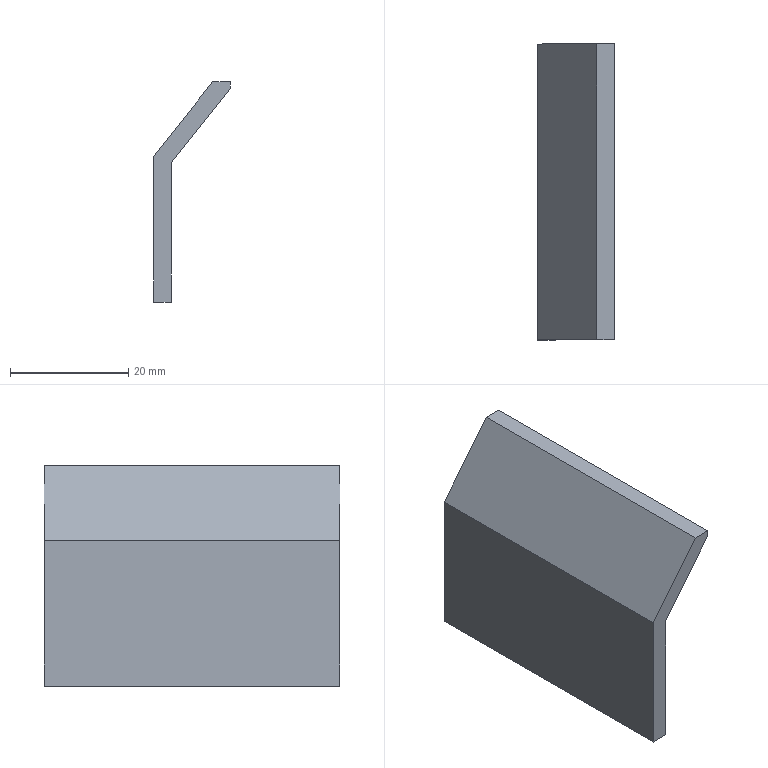Part | NX | features solid 2 | 1 solid | 9 faces | box 13 x 50 x 37.219 mm | volume 6106 mm3 | plane 9
STEP:
#1=CARTESIAN_POINT('',(-1175.,-370.,-87.));
#2=VERTEX_POINT('',#1);
#3=CARTESIAN_POINT('',(-1172.,-370.,-87.));
#4=VERTEX_POINT('',#3);
#5=CARTESIAN_POINT('',(-1175.,-370.,-87.));
#6=DIRECTION('',(1.,0.,0.));
#7=VECTOR('',#6,1000.);
#8=LINE('',#5,#7);
#9=EDGE_CURVE('',#2,#4,#8,.T.);
#10=ORIENTED_EDGE('',*,*,#9,.T.);
#11=CARTESIAN_POINT('',(-1172.,-420.,-87.));
#12=VERTEX_POINT('',#11);
#13=CARTESIAN_POINT('',(-1172.,-445.,-87.));
#14=DIRECTION('',(0.,1.,0.));
#15=VECTOR('',#14,1000.);
#16=LINE('',#13,#15);
#17=EDGE_CURVE('',#12,#4,#16,.T.);
#18=ORIENTED_EDGE('',*,*,#17,.F.);
#19=CARTESIAN_POINT('',(-1175.,-420.,-87.));
#20=VERTEX_POINT('',#19);
#21=CARTESIAN_POINT('',(-1175.,-420.,-87.));
#22=DIRECTION('',(1.,0.,0.));
#23=VECTOR('',#22,1000.);
#24=LINE('',#21,#23);
#25=EDGE_CURVE('',#20,#12,#24,.T.);
#26=ORIENTED_EDGE('',*,*,#25,.F.);
#27=CARTESIAN_POINT('',(-1175.,-445.,-87.));
#28=DIRECTION('',(0.,1.,0.));
#29=VECTOR('',#28,1000.);
#30=LINE('',#27,#29);
#31=EDGE_CURVE('',#20,#2,#30,.T.);
#32=ORIENTED_EDGE('',*,*,#31,.T.);
#33=EDGE_LOOP('',(#10,#18,#26,#32));
#34=FACE_BOUND('',#33,.T.);
#35=CARTESIAN_POINT('',(-1175.,-445.,-87.));
#36=DIRECTION('',(0.,0.,-1.));
#37=DIRECTION('',(-1.,0.,0.));
#38=AXIS2_PLACEMENT_3D('',#35,#36,#37);
#39=PLANE('',#38);
#40=ADVANCED_FACE('',(#34),#39,.T.);
#41=CARTESIAN_POINT('',(-1162.,-420.,-49.781));
#42=VERTEX_POINT('',#41);
#43=CARTESIAN_POINT('',(-1165.,-420.,-49.781));
#44=VERTEX_POINT('',#43);
#45=CARTESIAN_POINT('',(-1175.,-420.,-49.781));
#46=DIRECTION('',(-1.,0.,0.));
#47=VECTOR('',#46,1000.);
#48=LINE('',#45,#47);
#49=EDGE_CURVE('',#42,#44,#48,.T.);
#50=ORIENTED_EDGE('',*,*,#49,.T.);
#51=CARTESIAN_POINT('',(-1175.,-420.,-62.364));
#52=VERTEX_POINT('',#51);
#53=CARTESIAN_POINT('',(-1187.,-420.,-77.463));
#54=DIRECTION('',(0.6222,0.,0.7829));
#55=VECTOR('',#54,1000.);
#56=LINE('',#53,#55);
#57=EDGE_CURVE('',#52,#44,#56,.T.);
#58=ORIENTED_EDGE('',*,*,#57,.F.);
#59=CARTESIAN_POINT('',(-1175.,-420.,-87.));
#60=DIRECTION('',(0.,0.,1.));
#61=VECTOR('',#60,1000.);
#62=LINE('',#59,#61);
#63=EDGE_CURVE('',#20,#52,#62,.T.);
#64=ORIENTED_EDGE('',*,*,#63,.F.);
#65=ORIENTED_EDGE('',*,*,#25,.T.);
#66=CARTESIAN_POINT('',(-1172.,-420.,-63.411));
#67=VERTEX_POINT('',#66);
#68=CARTESIAN_POINT('',(-1172.,-420.,-87.));
#69=DIRECTION('',(0.,0.,1.));
#70=VECTOR('',#69,1000.);
#71=LINE('',#68,#70);
#72=EDGE_CURVE('',#12,#67,#71,.T.);
#73=ORIENTED_EDGE('',*,*,#72,.T.);
#74=CARTESIAN_POINT('',(-1162.,-420.,-50.828));
#75=VERTEX_POINT('',#74);
#76=CARTESIAN_POINT('',(-1160.826,-420.,-49.351));
#77=DIRECTION('',(-0.6222,0.,-0.7829));
#78=VECTOR('',#77,1000.);
#79=LINE('',#76,#78);
#80=EDGE_CURVE('',#75,#67,#79,.T.);
#81=ORIENTED_EDGE('',*,*,#80,.F.);
#82=CARTESIAN_POINT('',(-1162.,-420.,-87.));
#83=DIRECTION('',(0.,0.,1.));
#84=VECTOR('',#83,1000.);
#85=LINE('',#82,#84);
#86=EDGE_CURVE('',#75,#42,#85,.T.);
#87=ORIENTED_EDGE('',*,*,#86,.T.);
#88=EDGE_LOOP('',(#50,#58,#64,#65,#73,#81,#87));
#89=FACE_BOUND('',#88,.T.);
#90=CARTESIAN_POINT('',(-1175.,-420.,-87.));
#91=DIRECTION('',(0.,1.,0.));
#92=DIRECTION('',(0.,0.,-1.));
#93=AXIS2_PLACEMENT_3D('',#90,#91,#92);
#94=PLANE('',#93);
#95=ADVANCED_FACE('',(#89),#94,.F.);
#96=CARTESIAN_POINT('',(-1165.,-370.,-49.781));
#97=VERTEX_POINT('',#96);
#98=CARTESIAN_POINT('',(-1165.,-420.,-49.781));
#99=DIRECTION('',(0.,1.,0.));
#100=VECTOR('',#99,1000.);
#101=LINE('',#98,#100);
#102=EDGE_CURVE('',#44,#97,#101,.T.);
#103=ORIENTED_EDGE('',*,*,#102,.T.);
#104=CARTESIAN_POINT('',(-1175.,-370.,-62.364));
#105=VERTEX_POINT('',#104);
#106=CARTESIAN_POINT('',(-1163.174,-370.,-47.484));
#107=DIRECTION('',(0.6222,0.,0.7829));
#108=VECTOR('',#107,1000.);
#109=LINE('',#106,#108);
#110=EDGE_CURVE('',#105,#97,#109,.T.);
#111=ORIENTED_EDGE('',*,*,#110,.F.);
#112=CARTESIAN_POINT('',(-1175.,-420.,-62.364));
#113=DIRECTION('',(0.,1.,0.));
#114=VECTOR('',#113,1000.);
#115=LINE('',#112,#114);
#116=EDGE_CURVE('',#52,#105,#115,.T.);
#117=ORIENTED_EDGE('',*,*,#116,.F.);
#118=ORIENTED_EDGE('',*,*,#57,.T.);
#119=EDGE_LOOP('',(#103,#111,#117,#118));
#120=FACE_BOUND('',#119,.T.);
#121=CARTESIAN_POINT('',(-1163.174,-420.,-47.484));
#122=DIRECTION('',(-0.7829,0.,0.6222));
#123=DIRECTION('',(0.6222,0.,0.7829));
#124=AXIS2_PLACEMENT_3D('',#121,#122,#123);
#125=PLANE('',#124);
#126=ADVANCED_FACE('',(#120),#125,.T.);
#127=CARTESIAN_POINT('',(-1162.,-370.,-49.781));
#128=VERTEX_POINT('',#127);
#129=CARTESIAN_POINT('',(-1175.,-370.,-49.781));
#130=DIRECTION('',(1.,0.,0.));
#131=VECTOR('',#130,1000.);
#132=LINE('',#129,#131);
#133=EDGE_CURVE('',#97,#128,#132,.T.);
#134=ORIENTED_EDGE('',*,*,#133,.T.);
#135=CARTESIAN_POINT('',(-1162.,-370.,-50.828));
#136=VERTEX_POINT('',#135);
#137=CARTESIAN_POINT('',(-1162.,-370.,-47.));
#138=DIRECTION('',(0.,0.,1.));
#139=VECTOR('',#138,1000.);
#140=LINE('',#137,#139);
#141=EDGE_CURVE('',#136,#128,#140,.T.);
#142=ORIENTED_EDGE('',*,*,#141,.F.);
#143=CARTESIAN_POINT('',(-1172.,-370.,-63.411));
#144=VERTEX_POINT('',#143);
#145=CARTESIAN_POINT('',(-1184.651,-370.,-79.33));
#146=DIRECTION('',(-0.6222,0.,-0.7829));
#147=VECTOR('',#146,1000.);
#148=LINE('',#145,#147);
#149=EDGE_CURVE('',#136,#144,#148,.T.);
#150=ORIENTED_EDGE('',*,*,#149,.T.);
#151=CARTESIAN_POINT('',(-1172.,-370.,-87.));
#152=DIRECTION('',(0.,0.,1.));
#153=VECTOR('',#152,1000.);
#154=LINE('',#151,#153);
#155=EDGE_CURVE('',#4,#144,#154,.T.);
#156=ORIENTED_EDGE('',*,*,#155,.F.);
#157=ORIENTED_EDGE('',*,*,#9,.F.);
#158=CARTESIAN_POINT('',(-1175.,-370.,-87.));
#159=DIRECTION('',(0.,0.,1.));
#160=VECTOR('',#159,1000.);
#161=LINE('',#158,#160);
#162=EDGE_CURVE('',#2,#105,#161,.T.);
#163=ORIENTED_EDGE('',*,*,#162,.T.);
#164=ORIENTED_EDGE('',*,*,#110,.T.);
#165=EDGE_LOOP('',(#134,#142,#150,#156,#157,#163,#164));
#166=FACE_BOUND('',#165,.T.);
#167=CARTESIAN_POINT('',(-1175.,-370.,-87.));
#168=DIRECTION('',(0.,1.,0.));
#169=DIRECTION('',(0.,0.,-1.));
#170=AXIS2_PLACEMENT_3D('',#167,#168,#169);
#171=PLANE('',#170);
#172=ADVANCED_FACE('',(#166),#171,.T.);
#173=ORIENTED_EDGE('',*,*,#72,.F.);
#174=ORIENTED_EDGE('',*,*,#17,.T.);
#175=ORIENTED_EDGE('',*,*,#155,.T.);
#176=CARTESIAN_POINT('',(-1172.,-420.,-63.411));
#177=DIRECTION('',(0.,1.,0.));
#178=VECTOR('',#177,1000.);
#179=LINE('',#176,#178);
#180=EDGE_CURVE('',#67,#144,#179,.T.);
#181=ORIENTED_EDGE('',*,*,#180,.F.);
#182=EDGE_LOOP('',(#173,#174,#175,#181));
#183=FACE_BOUND('',#182,.T.);
#184=CARTESIAN_POINT('',(-1172.,-445.,-87.));
#185=DIRECTION('',(-1.,0.,0.));
#186=DIRECTION('',(0.,0.,1.));
#187=AXIS2_PLACEMENT_3D('',#184,#185,#186);
#188=PLANE('',#187);
#189=ADVANCED_FACE('',(#183),#188,.F.);
#190=ORIENTED_EDGE('',*,*,#116,.T.);
#191=ORIENTED_EDGE('',*,*,#162,.F.);
#192=ORIENTED_EDGE('',*,*,#31,.F.);
#193=ORIENTED_EDGE('',*,*,#63,.T.);
#194=EDGE_LOOP('',(#190,#191,#192,#193));
#195=FACE_BOUND('',#194,.T.);
#196=CARTESIAN_POINT('',(-1175.,-445.,-87.));
#197=DIRECTION('',(-1.,0.,0.));
#198=DIRECTION('',(0.,0.,1.));
#199=AXIS2_PLACEMENT_3D('',#196,#197,#198);
#200=PLANE('',#199);
#201=ADVANCED_FACE('',(#195),#200,.T.);
#202=ORIENTED_EDGE('',*,*,#180,.T.);
#203=ORIENTED_EDGE('',*,*,#149,.F.);
#204=CARTESIAN_POINT('',(-1162.,-420.,-50.828));
#205=DIRECTION('',(0.,1.,0.));
#206=VECTOR('',#205,1000.);
#207=LINE('',#204,#206);
#208=EDGE_CURVE('',#75,#136,#207,.T.);
#209=ORIENTED_EDGE('',*,*,#208,.F.);
#210=ORIENTED_EDGE('',*,*,#80,.T.);
#211=EDGE_LOOP('',(#202,#203,#209,#210));
#212=FACE_BOUND('',#211,.T.);
#213=CARTESIAN_POINT('',(-1160.826,-420.,-49.351));
#214=DIRECTION('',(-0.7829,0.,0.6222));
#215=DIRECTION('',(0.6222,0.,0.7829));
#216=AXIS2_PLACEMENT_3D('',#213,#214,#215);
#217=PLANE('',#216);
#218=ADVANCED_FACE('',(#212),#217,.F.);
#219=ORIENTED_EDGE('',*,*,#86,.F.);
#220=ORIENTED_EDGE('',*,*,#208,.T.);
#221=ORIENTED_EDGE('',*,*,#141,.T.);
#222=CARTESIAN_POINT('',(-1162.,-445.,-49.781));
#223=DIRECTION('',(0.,1.,0.));
#224=VECTOR('',#223,1000.);
#225=LINE('',#222,#224);
#226=EDGE_CURVE('',#42,#128,#225,.T.);
#227=ORIENTED_EDGE('',*,*,#226,.F.);
#228=EDGE_LOOP('',(#219,#220,#221,#227));
#229=FACE_BOUND('',#228,.T.);
#230=CARTESIAN_POINT('',(-1162.,-445.,-47.));
#231=DIRECTION('',(-1.,0.,0.));
#232=DIRECTION('',(0.,0.,1.));
#233=AXIS2_PLACEMENT_3D('',#230,#231,#232);
#234=PLANE('',#233);
#235=ADVANCED_FACE('',(#229),#234,.F.);
#236=ORIENTED_EDGE('',*,*,#49,.F.);
#237=ORIENTED_EDGE('',*,*,#226,.T.);
#238=ORIENTED_EDGE('',*,*,#133,.F.);
#239=ORIENTED_EDGE('',*,*,#102,.F.);
#240=EDGE_LOOP('',(#236,#237,#238,#239));
#241=FACE_BOUND('',#240,.T.);
#242=CARTESIAN_POINT('',(-1165.,-370.,-49.781));
#243=DIRECTION('',(0.,0.,-1.));
#244=DIRECTION('',(-1.,0.,0.));
#245=AXIS2_PLACEMENT_3D('',#242,#243,#244);
#246=PLANE('',#245);
#247=ADVANCED_FACE('',(#241),#246,.F.);
#248=CLOSED_SHELL('',(#40,#95,#126,#172,#189,#201,#218,#235,#247));
#249=MANIFOLD_SOLID_BREP('',#248);
#250=(LENGTH_UNIT()NAMED_UNIT(*)SI_UNIT(.MILLI.,.METRE.));
#251=UNCERTAINTY_MEASURE_WITH_UNIT(LENGTH_MEASURE(0.00001),#250,'','');
#252=(NAMED_UNIT(*)PLANE_ANGLE_UNIT()SI_UNIT($,.RADIAN.));
#253=(NAMED_UNIT(*)SI_UNIT($,.STERADIAN.)SOLID_ANGLE_UNIT());
#254=(GEOMETRIC_REPRESENTATION_CONTEXT(3)GLOBAL_UNCERTAINTY_ASSIGNED_CONTEXT((#251))GLOBAL_UNIT_ASSIGNED_CONTEXT((#250,#252,#253))REPRESENTATION_CONTEXT('',''));
#255=ADVANCED_BREP_SHAPE_REPRESENTATION('',(#249),#254);